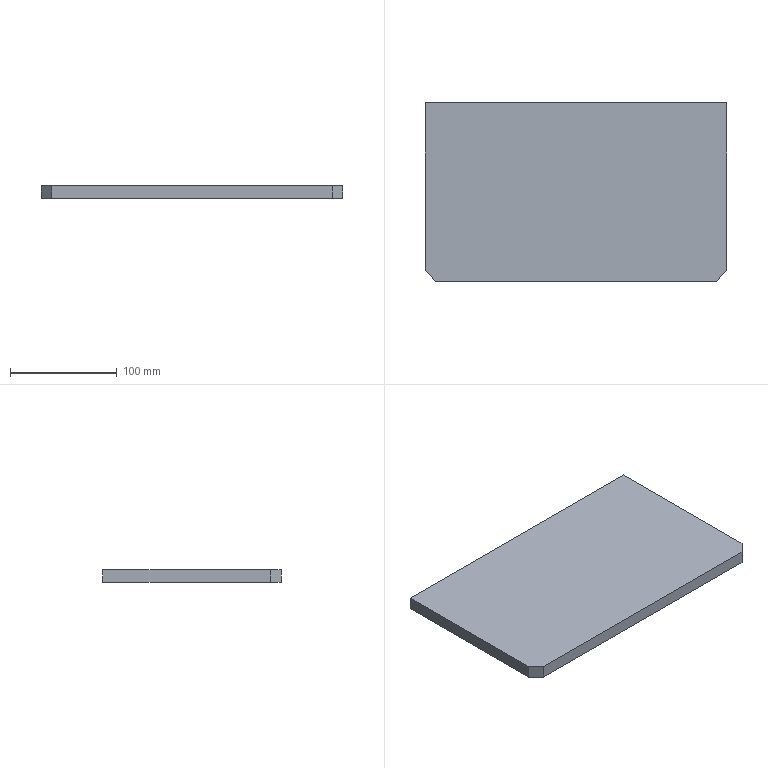Part | SolidWorks | features BaseBody 1 | 1 solid | 8 faces | box 282.5 x 167 x 12 mm | volume 564930 mm3 | plane 8
STEP:
#1=CARTESIAN_POINT('',(-141.25,82.,12.));
#2=VERTEX_POINT('',#1);
#3=CARTESIAN_POINT('',(-141.25,-75.,12.));
#4=VERTEX_POINT('',#3);
#5=CARTESIAN_POINT('',(-141.25,85.,12.));
#6=DIRECTION('',(0.,-1.,0.));
#7=VECTOR('',#6,1000.);
#8=LINE('',#5,#7);
#9=EDGE_CURVE('',#2,#4,#8,.T.);
#10=ORIENTED_EDGE('',*,*,#9,.F.);
#11=CARTESIAN_POINT('',(-141.25,82.,0.));
#12=VERTEX_POINT('',#11);
#13=CARTESIAN_POINT('',(-141.25,82.,12.));
#14=DIRECTION('',(0.,0.,-1.));
#15=VECTOR('',#14,1000.);
#16=LINE('',#13,#15);
#17=EDGE_CURVE('',#2,#12,#16,.T.);
#18=ORIENTED_EDGE('',*,*,#17,.T.);
#19=CARTESIAN_POINT('',(-141.25,-75.,0.));
#20=VERTEX_POINT('',#19);
#21=CARTESIAN_POINT('',(-141.25,85.,0.));
#22=DIRECTION('',(0.,-1.,0.));
#23=VECTOR('',#22,1000.);
#24=LINE('',#21,#23);
#25=EDGE_CURVE('',#12,#20,#24,.T.);
#26=ORIENTED_EDGE('',*,*,#25,.T.);
#27=CARTESIAN_POINT('',(-141.25,-75.,12.));
#28=DIRECTION('',(0.,0.,-1.));
#29=VECTOR('',#28,1000.);
#30=LINE('',#27,#29);
#31=EDGE_CURVE('',#4,#20,#30,.T.);
#32=ORIENTED_EDGE('',*,*,#31,.F.);
#33=EDGE_LOOP('',(#10,#18,#26,#32));
#34=FACE_OUTER_BOUND('',#33,.T.);
#35=CARTESIAN_POINT('',(-141.25,85.,12.));
#36=DIRECTION('',(1.,0.,0.));
#37=DIRECTION('',(0.,1.,0.));
#38=AXIS2_PLACEMENT_3D('',#35,#36,#37);
#39=PLANE('',#38);
#40=ADVANCED_FACE('',(#34),#39,.F.);
#41=CARTESIAN_POINT('',(-131.25,-85.,0.));
#42=VERTEX_POINT('',#41);
#43=CARTESIAN_POINT('',(-141.25,-75.,0.));
#44=DIRECTION('',(0.7071,-0.7071,0.));
#45=VECTOR('',#44,1000.);
#46=LINE('',#43,#45);
#47=EDGE_CURVE('',#20,#42,#46,.T.);
#48=ORIENTED_EDGE('',*,*,#47,.T.);
#49=CARTESIAN_POINT('',(-131.25,-85.,12.));
#50=VERTEX_POINT('',#49);
#51=CARTESIAN_POINT('',(-131.25,-85.,12.));
#52=DIRECTION('',(0.,0.,-1.));
#53=VECTOR('',#52,1000.);
#54=LINE('',#51,#53);
#55=EDGE_CURVE('',#50,#42,#54,.T.);
#56=ORIENTED_EDGE('',*,*,#55,.F.);
#57=CARTESIAN_POINT('',(-141.25,-75.,12.));
#58=DIRECTION('',(0.7071,-0.7071,0.));
#59=VECTOR('',#58,1000.);
#60=LINE('',#57,#59);
#61=EDGE_CURVE('',#4,#50,#60,.T.);
#62=ORIENTED_EDGE('',*,*,#61,.F.);
#63=ORIENTED_EDGE('',*,*,#31,.T.);
#64=EDGE_LOOP('',(#48,#56,#62,#63));
#65=FACE_OUTER_BOUND('',#64,.T.);
#66=CARTESIAN_POINT('',(-141.25,-75.,12.));
#67=DIRECTION('',(0.7071,0.7071,0.));
#68=DIRECTION('',(-0.7071,0.7071,0.));
#69=AXIS2_PLACEMENT_3D('',#66,#67,#68);
#70=PLANE('',#69);
#71=ADVANCED_FACE('',(#65),#70,.F.);
#72=CARTESIAN_POINT('',(131.25,-85.,0.));
#73=VERTEX_POINT('',#72);
#74=CARTESIAN_POINT('',(-131.25,-85.,0.));
#75=DIRECTION('',(1.,0.,0.));
#76=VECTOR('',#75,1000.);
#77=LINE('',#74,#76);
#78=EDGE_CURVE('',#42,#73,#77,.T.);
#79=ORIENTED_EDGE('',*,*,#78,.T.);
#80=CARTESIAN_POINT('',(131.25,-85.,12.));
#81=VERTEX_POINT('',#80);
#82=CARTESIAN_POINT('',(131.25,-85.,12.));
#83=DIRECTION('',(0.,0.,-1.));
#84=VECTOR('',#83,1000.);
#85=LINE('',#82,#84);
#86=EDGE_CURVE('',#81,#73,#85,.T.);
#87=ORIENTED_EDGE('',*,*,#86,.F.);
#88=CARTESIAN_POINT('',(-131.25,-85.,12.));
#89=DIRECTION('',(1.,0.,0.));
#90=VECTOR('',#89,1000.);
#91=LINE('',#88,#90);
#92=EDGE_CURVE('',#50,#81,#91,.T.);
#93=ORIENTED_EDGE('',*,*,#92,.F.);
#94=ORIENTED_EDGE('',*,*,#55,.T.);
#95=EDGE_LOOP('',(#79,#87,#93,#94));
#96=FACE_OUTER_BOUND('',#95,.T.);
#97=CARTESIAN_POINT('',(-131.25,-85.,12.));
#98=DIRECTION('',(0.,1.,0.));
#99=DIRECTION('',(0.,0.,1.));
#100=AXIS2_PLACEMENT_3D('',#97,#98,#99);
#101=PLANE('',#100);
#102=ADVANCED_FACE('',(#96),#101,.F.);
#103=CARTESIAN_POINT('',(141.25,-75.,0.));
#104=VERTEX_POINT('',#103);
#105=CARTESIAN_POINT('',(131.25,-85.,0.));
#106=DIRECTION('',(0.7071,0.7071,0.));
#107=VECTOR('',#106,1000.);
#108=LINE('',#105,#107);
#109=EDGE_CURVE('',#73,#104,#108,.T.);
#110=ORIENTED_EDGE('',*,*,#109,.T.);
#111=CARTESIAN_POINT('',(141.25,-75.,12.));
#112=VERTEX_POINT('',#111);
#113=CARTESIAN_POINT('',(141.25,-75.,12.));
#114=DIRECTION('',(0.,0.,-1.));
#115=VECTOR('',#114,1000.);
#116=LINE('',#113,#115);
#117=EDGE_CURVE('',#112,#104,#116,.T.);
#118=ORIENTED_EDGE('',*,*,#117,.F.);
#119=CARTESIAN_POINT('',(131.25,-85.,12.));
#120=DIRECTION('',(0.7071,0.7071,0.));
#121=VECTOR('',#120,1000.);
#122=LINE('',#119,#121);
#123=EDGE_CURVE('',#81,#112,#122,.T.);
#124=ORIENTED_EDGE('',*,*,#123,.F.);
#125=ORIENTED_EDGE('',*,*,#86,.T.);
#126=EDGE_LOOP('',(#110,#118,#124,#125));
#127=FACE_OUTER_BOUND('',#126,.T.);
#128=CARTESIAN_POINT('',(131.25,-85.,12.));
#129=DIRECTION('',(-0.7071,0.7071,0.));
#130=DIRECTION('',(-0.7071,-0.7071,0.));
#131=AXIS2_PLACEMENT_3D('',#128,#129,#130);
#132=PLANE('',#131);
#133=ADVANCED_FACE('',(#127),#132,.F.);
#134=CARTESIAN_POINT('',(141.25,82.,0.));
#135=VERTEX_POINT('',#134);
#136=CARTESIAN_POINT('',(141.25,85.,0.));
#137=DIRECTION('',(0.,1.,0.));
#138=VECTOR('',#137,1000.);
#139=LINE('',#136,#138);
#140=EDGE_CURVE('',#104,#135,#139,.T.);
#141=ORIENTED_EDGE('',*,*,#140,.T.);
#142=CARTESIAN_POINT('',(141.25,82.,12.));
#143=VERTEX_POINT('',#142);
#144=CARTESIAN_POINT('',(141.25,82.,12.));
#145=DIRECTION('',(0.,0.,1.));
#146=VECTOR('',#145,1000.);
#147=LINE('',#144,#146);
#148=EDGE_CURVE('',#135,#143,#147,.T.);
#149=ORIENTED_EDGE('',*,*,#148,.T.);
#150=CARTESIAN_POINT('',(141.25,85.,12.));
#151=DIRECTION('',(0.,1.,0.));
#152=VECTOR('',#151,1000.);
#153=LINE('',#150,#152);
#154=EDGE_CURVE('',#112,#143,#153,.T.);
#155=ORIENTED_EDGE('',*,*,#154,.F.);
#156=ORIENTED_EDGE('',*,*,#117,.T.);
#157=EDGE_LOOP('',(#141,#149,#155,#156));
#158=FACE_OUTER_BOUND('',#157,.T.);
#159=CARTESIAN_POINT('',(141.25,85.,12.));
#160=DIRECTION('',(-1.,0.,0.));
#161=DIRECTION('',(0.,-1.,0.));
#162=AXIS2_PLACEMENT_3D('',#159,#160,#161);
#163=PLANE('',#162);
#164=ADVANCED_FACE('',(#158),#163,.F.);
#165=CARTESIAN_POINT('',(0.,82.,12.));
#166=DIRECTION('',(1.,0.,0.));
#167=VECTOR('',#166,1000.);
#168=LINE('',#165,#167);
#169=EDGE_CURVE('',#2,#143,#168,.T.);
#170=ORIENTED_EDGE('',*,*,#169,.F.);
#171=ORIENTED_EDGE('',*,*,#9,.T.);
#172=ORIENTED_EDGE('',*,*,#61,.T.);
#173=ORIENTED_EDGE('',*,*,#92,.T.);
#174=ORIENTED_EDGE('',*,*,#123,.T.);
#175=ORIENTED_EDGE('',*,*,#154,.T.);
#176=EDGE_LOOP('',(#170,#171,#172,#173,#174,#175));
#177=FACE_OUTER_BOUND('',#176,.T.);
#178=CARTESIAN_POINT('',(0.,0.,12.));
#179=DIRECTION('',(0.,0.,1.));
#180=DIRECTION('',(1.,0.,0.));
#181=AXIS2_PLACEMENT_3D('',#178,#179,#180);
#182=PLANE('',#181);
#183=ADVANCED_FACE('',(#177),#182,.T.);
#184=ORIENTED_EDGE('',*,*,#25,.F.);
#185=CARTESIAN_POINT('',(0.,82.,0.));
#186=DIRECTION('',(1.,0.,0.));
#187=VECTOR('',#186,1000.);
#188=LINE('',#185,#187);
#189=EDGE_CURVE('',#12,#135,#188,.T.);
#190=ORIENTED_EDGE('',*,*,#189,.T.);
#191=ORIENTED_EDGE('',*,*,#140,.F.);
#192=ORIENTED_EDGE('',*,*,#109,.F.);
#193=ORIENTED_EDGE('',*,*,#78,.F.);
#194=ORIENTED_EDGE('',*,*,#47,.F.);
#195=EDGE_LOOP('',(#184,#190,#191,#192,#193,#194));
#196=FACE_OUTER_BOUND('',#195,.T.);
#197=CARTESIAN_POINT('',(0.,0.,0.));
#198=DIRECTION('',(0.,0.,1.));
#199=DIRECTION('',(1.,0.,0.));
#200=AXIS2_PLACEMENT_3D('',#197,#198,#199);
#201=PLANE('',#200);
#202=ADVANCED_FACE('',(#196),#201,.F.);
#203=ORIENTED_EDGE('',*,*,#169,.T.);
#204=ORIENTED_EDGE('',*,*,#148,.F.);
#205=ORIENTED_EDGE('',*,*,#189,.F.);
#206=ORIENTED_EDGE('',*,*,#17,.F.);
#207=EDGE_LOOP('',(#203,#204,#205,#206));
#208=FACE_OUTER_BOUND('',#207,.T.);
#209=CARTESIAN_POINT('',(441.75,82.,6.));
#210=DIRECTION('',(0.,-1.,0.));
#211=DIRECTION('',(0.,0.,-1.));
#212=AXIS2_PLACEMENT_3D('',#209,#210,#211);
#213=PLANE('',#212);
#214=ADVANCED_FACE('',(#208),#213,.F.);
#215=CLOSED_SHELL('',(#40,#71,#102,#133,#164,#183,#202,#214));
#216=MANIFOLD_SOLID_BREP('',#215);
#217=CARTESIAN_POINT('',(0.,0.,0.));
#218=DIRECTION('',(0.,0.,1.));
#219=DIRECTION('',(1.,0.,0.));
#220=AXIS2_PLACEMENT_3D('',#217,#218,#219);
#221=(LENGTH_UNIT()NAMED_UNIT(*)SI_UNIT(.MILLI.,.METRE.));
#222=UNCERTAINTY_MEASURE_WITH_UNIT(LENGTH_MEASURE(0.00001),#221,'','');
#223=(NAMED_UNIT(*)PLANE_ANGLE_UNIT()SI_UNIT($,.RADIAN.));
#224=(NAMED_UNIT(*)SI_UNIT($,.STERADIAN.)SOLID_ANGLE_UNIT());
#225=(GEOMETRIC_REPRESENTATION_CONTEXT(3)GLOBAL_UNCERTAINTY_ASSIGNED_CONTEXT((#222))GLOBAL_UNIT_ASSIGNED_CONTEXT((#221,#223,#224))REPRESENTATION_CONTEXT('',''));
#226=ADVANCED_BREP_SHAPE_REPRESENTATION('',(#216,#220),#225);